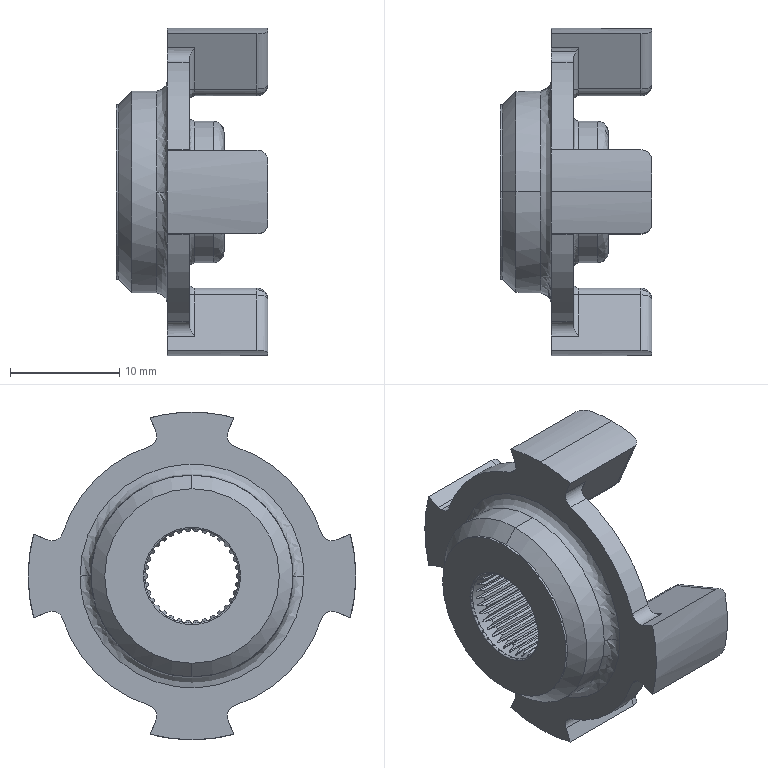Part | STEP file | TQ-DD-1105-TH SAP_405441541010 Default | 1 solid | 306 faces | box 13.9 x 30 x 30 mm | volume 3137 mm3 | cylinder 176 | plane 84 | spline 40 | cone 6 | commonest cylinder face diameters 0.262 x86 8.183 x34 2 x28 1 x8 17.7 x5 30 x5